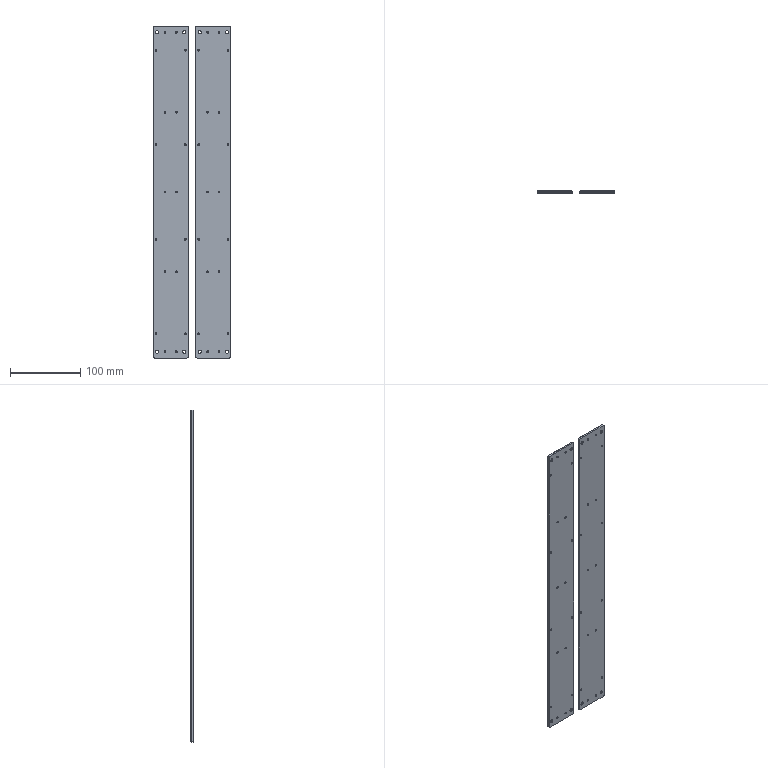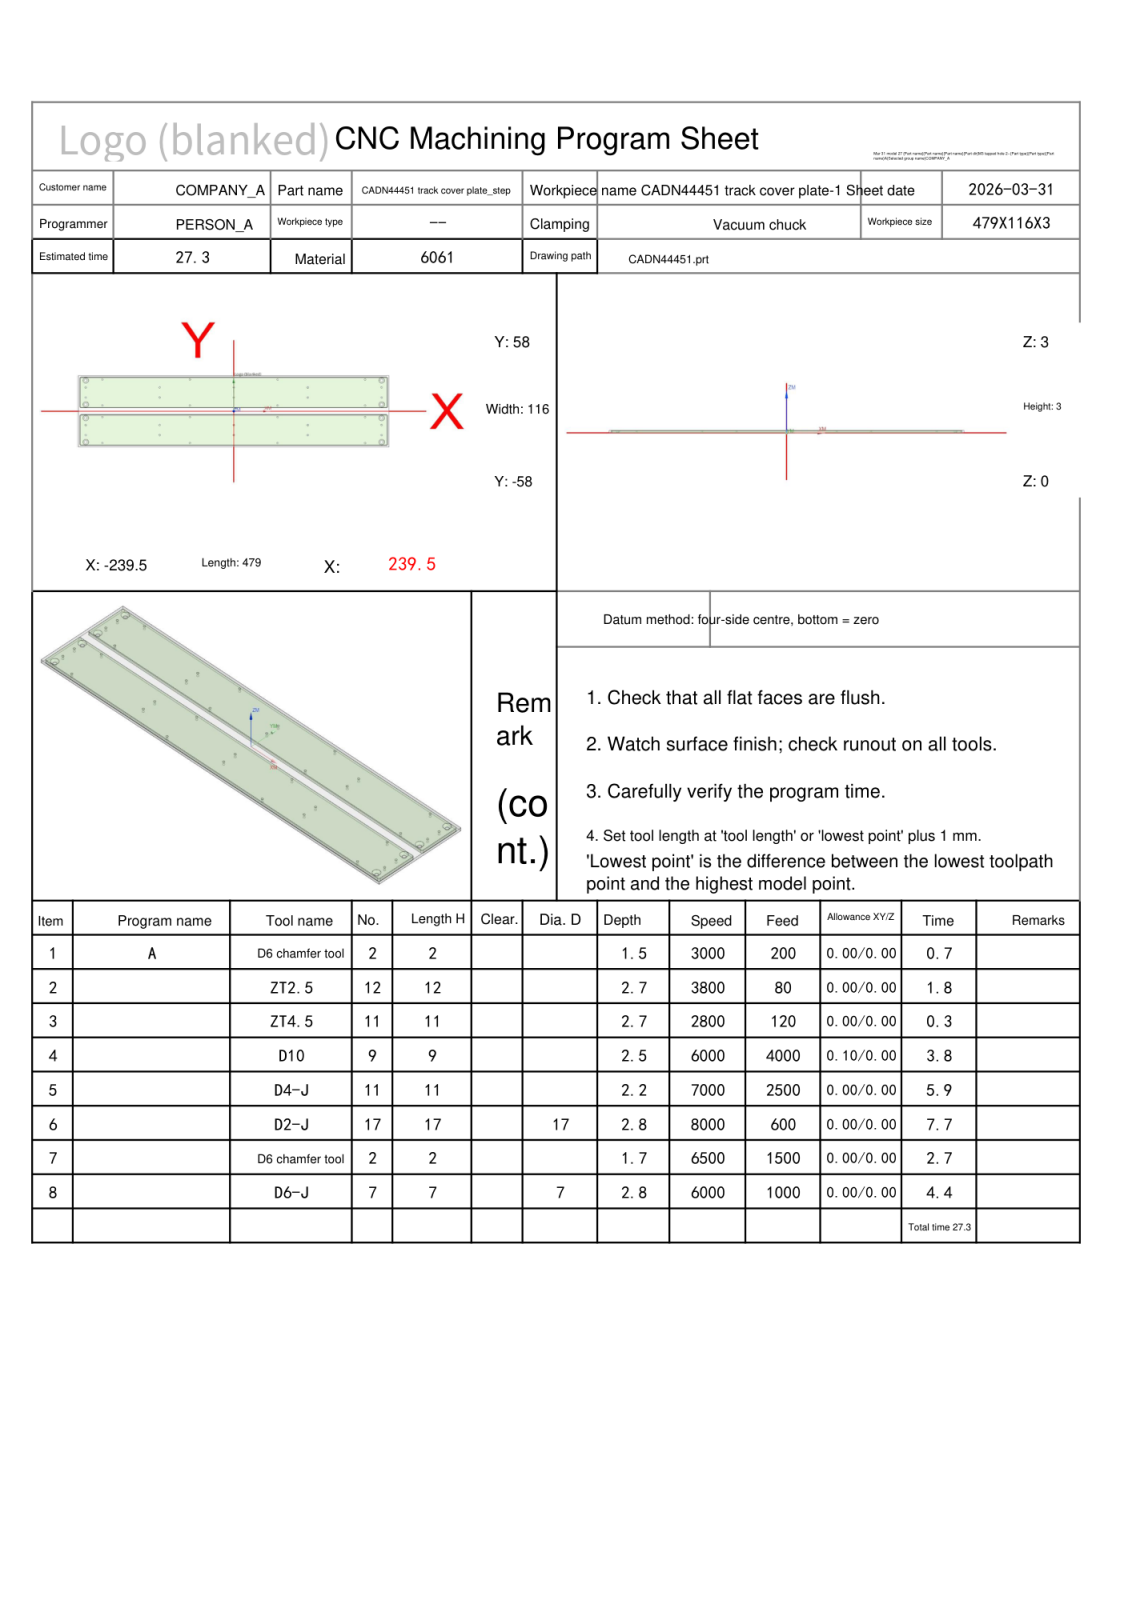NC program | NX | posted by the shop | part box 111 x 3 x 474 mm
Lines 279 to 1191 of 17996:
N5 T11 M06
(D4-J  D=4. R=0. H=11 ce=0.00 di=0.00)
G00 G90 G54 X226.061 Y51.525 M03 S7000
G43 H11 Z23.
M08
Z4.5
G01 X225.989 Y51.441 Z4.494 F2500.
X225.822 Y51.174 Z4.478
X225.661 Y50.807 Z4.457
X225.561 Y50.419 Z4.436
X225.526 Y50.019 Z4.415
X225.555 Y49.619 Z4.394
X225.649 Y49.229 Z4.373
X225.804 Y48.859 Z4.352
X226.017 Y48.52 Z4.331
X226.283 Y48.219 Z4.31
X226.593 Y47.965 Z4.289
X226.94 Y47.764 Z4.268
X227.232 Y47.648 Z4.251
X227.53 Y47.571 Z4.235
X227.835 Y47.531 Z4.219
X228.143 Y47.53 Z4.203
X228.455 Y47.568 Z4.186
X228.861 Y47.68 Z4.164
X229.242 Y47.86 Z4.142
X229.587 Y48.102 Z4.12
X229.886 Y48.399 Z4.098
X230.131 Y48.742 Z4.076
X230.313 Y49.121 Z4.054
X230.429 Y49.526 Z4.032
X230.474 Y49.945 Z4.01
X230.447 Y50.366 Z3.988
X230.35 Y50.776 Z3.965
X230.184 Y51.163 Z3.943
X230.019 Y51.431 Z3.927
X229.734 Y51.766 Z3.904
X229.393 Y52.045 Z3.881
X229.009 Y52.259 Z3.858
X228.592 Y52.402 Z3.835
X228.157 Y52.469 Z3.812
X227.843 Z3.795
X227.41 Y52.403 Z3.772
X226.996 Y52.262 Z3.749
X226.613 Y52.049 Z3.726
X226.274 Y51.773 Z3.703
X225.989 Y51.441 Z3.68
X225.822 Y51.174 Z3.664
X225.661 Y50.807 Z3.643
X225.561 Y50.419 Z3.622
X225.526 Y50.019 Z3.601
X225.555 Y49.619 Z3.58
X225.649 Y49.229 Z3.559
X225.804 Y48.859 Z3.538
X226.017 Y48.52 Z3.517
X226.283 Y48.219 Z3.496
X226.593 Y47.965 Z3.475
X226.94 Y47.764 Z3.454
X227.232 Y47.648 Z3.437
X227.53 Y47.571 Z3.421
X227.835 Y47.531 Z3.405
X228.143 Y47.53 Z3.389
X228.455 Y47.568 Z3.372
X228.861 Y47.68 Z3.35
X229.242 Y47.86 Z3.328
X229.587 Y48.102 Z3.306
X229.886 Y48.399 Z3.284
X230.131 Y48.742 Z3.262
X230.313 Y49.121 Z3.24
X230.429 Y49.526 Z3.218
X230.474 Y49.945 Z3.196
X230.447 Y50.366 Z3.174
X230.35 Y50.776 Z3.152
X230.184 Y51.163 Z3.129
X230.019 Y51.431 Z3.113
X229.734 Y51.766 Z3.09
X229.393 Y52.045 Z3.067
X229.009 Y52.259 Z3.044
X228.592 Y52.402 Z3.021
X228.157 Y52.469 Z2.998
X228. Z2.989
G03 X225.531 Y50. I0.0 J-2.469
X228. Y47.531 I2.469 J0.0
X230.469 Y50. I0.0 J2.469
X228. Y52.469 I-2.469 J0.0
G01 X227.94 Y52.463 Z2.984
X227.879 Y52.456 Z2.979
G03 X225.541 Y50. I.121 J-2.456
X228. Y47.541 I2.459 J0.0
X230.459 Y50. I0.0 J2.459
X228. Y52.459 I-2.459 J0.0
G01 X227.94 Y52.453 Z2.973
X227.879 Y52.445 Z2.968
G03 X225.552 Y50. I.121 J-2.445
X228. Y47.552 I2.448 J0.0
X230.448 Y50. I0.0 J2.448
X228. Y52.448 I-2.448 J0.0
G01 X227.94 Y52.442 Z2.963
X227.879 Y52.435 Z2.958
G03 X225.562 Y50. I.121 J-2.435
X228. Y47.562 I2.438 J0.0
X230.438 Y50. I0.0 J2.438
X228. Y52.438 I-2.438 J0.0
G01 X227.94 Y52.432 Z2.952
X227.879 Y52.424 Z2.947
G03 X225.573 Y50. I.121 J-2.424
X228. Y47.573 I2.427 J0.0
X230.427 Y50. I0.0 J2.427
X228. Y52.427 I-2.427 J0.0
G01 X227.94 Y52.421 Z2.942
X227.879 Y52.413 Z2.936
G03 X225.584 Y50. I.121 J-2.413
X228. Y47.584 I2.416 J0.0
X230.416 Y50. I0.0 J2.416
X228. Y52.416 I-2.416 J0.0
G01 X227.94 Y52.41 Z2.931
X227.879 Y52.403 Z2.926
G03 X225.594 Y50. I.121 J-2.403
X228. Y47.594 I2.406 J0.0
X230.406 Y50. I0.0 J2.406
X228. Y52.406 I-2.406 J0.0
G01 X227.94 Y52.4 Z2.92
X227.879 Y52.392 Z2.915
G03 X225.605 Y50. I.121 J-2.392
X228. Y47.605 I2.395 J0.0
X230.395 Y50. I0.0 J2.395
X228. Y52.395 I-2.395 J0.0
G01 X227.94 Y52.389 Z2.91
X227.879 Y52.381 Z2.905
G03 X225.615 Y50. I.121 J-2.381
X228. Y47.615 I2.385 J0.0
X230.385 Y50. I0.0 J2.385
X228. Y52.385 I-2.385 J0.0
G01 X227.94 Y52.378 Z2.899
X227.879 Y52.371 Z2.894
G03 X225.626 Y50. I.121 J-2.371
X228. Y47.626 I2.374 J0.0
X230.374 Y50. I0.0 J2.374
X228. Y52.374 I-2.374 J0.0
G01 X227.94 Y52.368 Z2.889
X227.879 Y52.36 Z2.883
G03 X225.637 Y50. I.121 J-2.36
X228. Y47.637 I2.363 J0.0
X230.363 Y50. I0.0 J2.363
X228. Y52.363 I-2.363 J0.0
G01 X227.94 Y52.357 Z2.878
X227.879 Y52.35 Z2.873
G03 X225.647 Y50. I.121 J-2.35
X228. Y47.647 I2.353 J0.0
X230.353 Y50. I0.0 J2.353
X228. Y52.353 I-2.353 J0.0
G01 X227.94 Y52.347 Z2.867
X227.879 Y52.339 Z2.862
G03 X225.658 Y50. I.121 J-2.339
X228. Y47.658 I2.342 J0.0
X230.342 Y50. I0.0 J2.342
X228. Y52.342 I-2.342 J0.0
G01 X227.94 Y52.336 Z2.857
X227.879 Y52.328 Z2.852
G03 X225.668 Y50. I.121 J-2.328
X228. Y47.668 I2.332 J0.0
X230.332 Y50. I0.0 J2.332
X228. Y52.332 I-2.332 J0.0
G01 X227.94 Y52.325 Z2.846
X227.879 Y52.318 Z2.841
G03 X225.679 Y50. I.121 J-2.318
X228. Y47.679 I2.321 J0.0
X230.321 Y50. I0.0 J2.321
X228. Y52.321 I-2.321 J0.0
G01 X227.94 Y52.315 Z2.836
X227.879 Y52.307 Z2.83
G03 X225.69 Y50. I.121 J-2.307
X228. Y47.69 I2.31 J0.0
X230.31 Y50. I0.0 J2.31
X228. Y52.31 I-2.31 J0.0
G01 X227.94 Y52.304 Z2.825
X227.879 Y52.297 Z2.82
G03 X225.7 Y50. I.121 J-2.297
X228. Y47.7 I2.3 J0.0
X230.3 Y50. I0.0 J2.3
X228. Y52.3 I-2.3 J0.0
G01 X227.94 Y52.294 Z2.814
X227.879 Y52.286 Z2.809
G03 X225.711 Y50. I.121 J-2.286
X228. Y47.711 I2.289 J0.0
X230.289 Y50. I0.0 J2.289
X228. Y52.289 I-2.289 J0.0
G01 X227.94 Y52.283 Z2.804
X227.879 Y52.275 Z2.798
G03 X225.722 Y50. I.121 J-2.275
X228. Y47.722 I2.278 J0.0
X230.278 Y50. I0.0 J2.278
X228. Y52.278 I-2.278 J0.0
G01 X227.94 Y52.272 Z2.793
X227.879 Y52.265 Z2.788
G03 X225.732 Y50. I.121 J-2.265
X228. Y47.732 I2.268 J0.0
X230.268 Y50. I0.0 J2.268
X228. Y52.268 I-2.268 J0.0
G01 X227.94 Y52.262 Z2.783
X227.879 Y52.254 Z2.777
G03 X225.743 Y50. I.121 J-2.254
X228. Y47.743 I2.257 J0.0
X230.257 Y50. I0.0 J2.257
X228. Y52.257 I-2.257 J0.0
G01 X227.94 Y52.251 Z2.772
X227.879 Y52.243 Z2.767
G03 X225.753 Y50. I.121 J-2.243
X228. Y47.753 I2.247 J0.0
X230.247 Y50. I0.0 J2.247
X228. Y52.247 I-2.247 J0.0
G01 X227.94 Y52.241 Z2.761
X227.879 Y52.233 Z2.756
G03 X225.764 Y50. I.121 J-2.233
X228. Y47.764 I2.236 J0.0
X230.236 Y50. I0.0 J2.236
X228. Y52.236 I-2.236 J0.0
G01 X227.94 Y52.23 Z2.751
X227.879 Y52.222 Z2.745
G03 X225.775 Y50. I.121 J-2.222
X228. Y47.775 I2.225 J0.0
X230.225 Y50. I0.0 J2.225
X228. Y52.225 I-2.225 J0.0
G01 X227.94 Y52.219 Z2.74
X227.879 Y52.212 Z2.735
G03 X225.785 Y50. I.121 J-2.212
X228. Y47.785 I2.215 J0.0
X230.215 Y50. I0.0 J2.215
X228. Y52.215 I-2.215 J0.0
G01 X227.94 Y52.209 Z2.73
X227.879 Y52.201 Z2.724
G03 X225.796 Y50. I.121 J-2.201
X228. Y47.796 I2.204 J0.0
X230.204 Y50. I0.0 J2.204
X228. Y52.204 I-2.204 J0.0
G01 X227.94 Y52.198 Z2.719
X227.879 Y52.19 Z2.714
G03 X225.806 Y50. I.121 J-2.19
X228. Y47.806 I2.194 J0.0
X230.194 Y50. I0.0 J2.194
X228. Y52.194 I-2.194 J0.0
G01 X227.94 Y52.187 Z2.708
X227.879 Y52.18 Z2.703
G03 X225.817 Y50. I.121 J-2.18
X228. Y47.817 I2.183 J0.0
X230.183 Y50. I0.0 J2.183
X228. Y52.183 I-2.183 J0.0
G01 X227.94 Y52.177 Z2.698
X227.879 Y52.169 Z2.692
G03 X225.828 Y50. I.121 J-2.169
X228. Y47.828 I2.172 J0.0
X230.172 Y50. I0.0 J2.172
X228. Y52.172 I-2.172 J0.0
G01 X227.94 Y52.166 Z2.687
X227.879 Y52.158 Z2.682
G03 X225.838 Y50. I.121 J-2.158
X228. Y47.838 I2.162 J0.0
X230.162 Y50. I0.0 J2.162
X228. Y52.162 I-2.162 J0.0
G01 X227.94 Y52.156 Z2.676
X227.879 Y52.148 Z2.671
G03 X225.849 Y50. I.121 J-2.148
X228. Y47.849 I2.151 J0.0
X230.151 Y50. I0.0 J2.151
X228. Y52.151 I-2.151 J0.0
G01 X227.94 Y52.145 Z2.666
X227.879 Y52.137 Z2.661
G03 X225.859 Y50. I.121 J-2.137
X228. Y47.859 I2.141 J0.0
X230.141 Y50. I0.0 J2.141
X228. Y52.141 I-2.141 J0.0
G01 X227.94 Y52.134 Z2.655
X227.879 Y52.127 Z2.65
G03 X225.87 Y50. I.121 J-2.127
X228. Y47.87 I2.13 J0.0
X230.13 Y50. I0.0 J2.13
X228. Y52.13 I-2.13 J0.0
G01 X227.94 Y52.124 Z2.645
X227.879 Y52.116 Z2.639
G03 X225.881 Y50. I.121 J-2.116
X228. Y47.881 I2.119 J0.0
X230.119 Y50. I0.0 J2.119
X228. Y52.119 I-2.119 J0.0
G01 X227.94 Y52.113 Z2.634
X227.879 Y52.105 Z2.629
G03 X225.891 Y50. I.121 J-2.105
X228. Y47.891 I2.109 J0.0
X230.109 Y50. I0.0 J2.109
X228. Y52.109 I-2.109 J0.0
G01 X227.94 Y52.103 Z2.623
X227.879 Y52.095 Z2.618
G03 X225.902 Y50. I.121 J-2.095
X228. Y47.902 I2.098 J0.0
X230.098 Y50. I0.0 J2.098
X228. Y52.098 I-2.098 J0.0
G01 X227.94 Y52.092 Z2.613
X227.879 Y52.084 Z2.608
G03 X225.912 Y50. I.121 J-2.084
X228. Y47.912 I2.088 J0.0
X230.088 Y50. I0.0 J2.088
X228. Y52.088 I-2.088 J0.0
G01 X227.94 Y52.081 Z2.602
X227.879 Y52.073 Z2.597
G03 X225.923 Y50. I.121 J-2.073
X228. Y47.923 I2.077 J0.0
X230.077 Y50. I0.0 J2.077
X228. Y52.077 I-2.077 J0.0
G01 X227.94 Y52.071 Z2.592
X227.879 Y52.063 Z2.586
G03 X225.934 Y50. I.121 J-2.063
X228. Y47.934 I2.066 J0.0
X230.066 Y50. I0.0 J2.066
X228. Y52.066 I-2.066 J0.0
G01 X227.94 Y52.06 Z2.581
X227.879 Y52.052 Z2.576
G03 X225.944 Y50. I.121 J-2.052
X228. Y47.944 I2.056 J0.0
X230.056 Y50. I0.0 J2.056
X228. Y52.056 I-2.056 J0.0
G01 X227.94 Y52.05 Z2.57
X227.879 Y52.042 Z2.565
G03 X225.955 Y50. I.121 J-2.042
X228. Y47.955 I2.045 J0.0
X230.045 Y50. I0.0 J2.045
X228. Y52.045 I-2.045 J0.0
G01 X227.94 Y52.039 Z2.56
X227.879 Y52.031 Z2.555
G03 X225.965 Y50. I.121 J-2.031
X228. Y47.965 I2.035 J0.0
X230.035 Y50. I0.0 J2.035
X228. Y52.035 I-2.035 J0.0
G01 X227.94 Y52.028 Z2.549
X227.879 Y52.02 Z2.544
G03 X225.976 Y50. I.121 J-2.02
X228. Y47.976 I2.024 J0.0
X230.024 Y50. I0.0 J2.024
X228. Y52.024 I-2.024 J0.0
G01 X227.94 Y52.018 Z2.539
X227.879 Y52.01 Z2.533
G03 X225.987 Y50. I.121 J-2.01
X228. Y47.987 I2.013 J0.0
X230.013 Y50. I0.0 J2.013
X228. Y52.013 I-2.013 J0.0
G01 X227.94 Y52.007 Z2.528
X227.879 Y51.999 Z2.523
G03 X225.997 Y50. I.121 J-1.999
X228. Y47.997 I2.003 J0.0
X230.003 Y50. I0.0 J2.003
X228. Y52.003 I-2.003 J0.0
G01 X227.94 Y51.996 Z2.517
X227.879 Y51.988 Z2.512
G03 X226.008 Y50. I.121 J-1.988
X228. Y48.008 I1.992 J0.0
X229.992 Y50. I0.0 J1.992
X228. Y51.992 I-1.992 J0.0
G01 X227.94 Y51.986 Z2.507
X227.879 Y51.978 Z2.501
G03 X226.019 Y50. I.121 J-1.978
X228. Y48.019 I1.981 J0.0
X229.981 Y50. I0.0 J1.981
X228. Y51.981 I-1.981 J0.0
G01 X227.94 Y51.975 Z2.496
X227.879 Y51.967 Z2.491
G03 X226.029 Y50. I.121 J-1.967
X228. Y48.029 I1.971 J0.0
X229.971 Y50. I0.0 J1.971
X228. Y51.971 I-1.971 J0.0
G01 X227.94 Y51.965 Z2.486
X227.879 Y51.957 Z2.48
G03 X226.04 Y50. I.121 J-1.957
X228. Y48.04 I1.96 J0.0
X229.96 Y50. I0.0 J1.96
X228. Y51.96 I-1.96 J0.0
G01 X227.94 Y51.954 Z2.475
X227.879 Y51.946 Z2.47
G03 X226.05 Y50. I.121 J-1.946
X228. Y48.05 I1.95 J0.0
X229.95 Y50. I0.0 J1.95
X228. Y51.95 I-1.95 J0.0
G01 X227.94 Y51.943 Z2.464
X227.88 Y51.935 Z2.459
G03 X226.061 Y50. I.12 J-1.935
X228. Y48.061 I1.939 J0.0
X229.939 Y50. I0.0 J1.939
X228. Y51.939 I-1.939 J0.0
G01 X227.94 Y51.933 Z2.454
X227.88 Y51.925 Z2.448
G03 X226.072 Y50. I.12 J-1.925
X228. Y48.072 I1.928 J0.0
X229.928 Y50. I0.0 J1.928
X228. Y51.928 I-1.928 J0.0
G01 X227.94 Y51.922 Z2.443
X227.88 Y51.914 Z2.438
G03 X226.082 Y50. I.12 J-1.914
X228. Y48.082 I1.918 J0.0
X229.918 Y50. I0.0 J1.918
X228. Y51.918 I-1.918 J0.0
G01 X227.94 Y51.912 Z2.433
X227.88 Y51.903 Z2.427
G03 X226.093 Y50. I.12 J-1.903
X228. Y48.093 I1.907 J0.0
X229.907 Y50. I0.0 J1.907
X228. Y51.907 I-1.907 J0.0
G01 X227.94 Y51.901 Z2.422
X227.88 Y51.893 Z2.417
G03 X226.103 Y50. I.12 J-1.893
X228. Y48.103 I1.897 J0.0
X229.897 Y50. I0.0 J1.897
X228. Y51.897 I-1.897 J0.0
G01 X227.94 Y51.89 Z2.411
X227.88 Y51.882 Z2.406
G03 X226.114 Y50. I.12 J-1.882
X228. Y48.114 I1.886 J0.0
X229.886 Y50. I0.0 J1.886
X228. Y51.886 I-1.886 J0.0
G01 X227.94 Y51.88 Z2.401
X227.88 Y51.872 Z2.395
G03 X226.125 Y50. I.12 J-1.872
X228. Y48.125 I1.875 J0.0
X229.875 Y50. I0.0 J1.875
X228. Y51.875 I-1.875 J0.0
G01 X227.94 Y51.869 Z2.39
X227.88 Y51.861 Z2.385
G03 X226.135 Y50. I.12 J-1.861
X228. Y48.135 I1.865 J0.0
X229.865 Y50. I0.0 J1.865
X228. Y51.865 I-1.865 J0.0
G01 X227.94 Y51.859 Z2.38
X227.88 Y51.85 Z2.374
G03 X226.146 Y50. I.12 J-1.85
X228. Y48.146 I1.854 J0.0
X229.854 Y50. I0.0 J1.854
X228. Y51.854 I-1.854 J0.0
G01 X227.94 Y51.848 Z2.369
X227.88 Y51.84 Z2.364
G03 X226.156 Y50. I.12 J-1.84
X228. Y48.156 I1.844 J0.0
X229.844 Y50. I0.0 J1.844
X228. Y51.844 I-1.844 J0.0
G01 X227.94 Y51.837 Z2.358
X227.88 Y51.829 Z2.353
G03 X226.167 Y50. I.12 J-1.829
X228. Y48.167 I1.833 J0.0
X229.833 Y50. I0.0 J1.833
X228. Y51.833 I-1.833 J0.0
G01 X227.94 Y51.827 Z2.348
X227.88 Y51.818 Z2.342
G03 X226.178 Y50. I.12 J-1.818
X228. Y48.178 I1.822 J0.0
X229.822 Y50. I0.0 J1.822
X228. Y51.822 I-1.822 J0.0
G01 X227.94 Y51.816 Z2.337
X227.88 Y51.808 Z2.332
G03 X226.188 Y50. I.12 J-1.808
X228. Y48.188 I1.812 J0.0
X229.812 Y50. I0.0 J1.812
X228. Y51.812 I-1.812 J0.0
G01 X227.94 Y51.805 Z2.326
X227.88 Y51.797 Z2.321
G03 X226.199 Y50. I.12 J-1.797
X228. Y48.199 I1.801 J0.0
X229.801 Y50. I0.0 J1.801
X228. Y51.801 I-1.801 J0.0
G01 X227.94 Y51.795 Z2.316
X227.88 Y51.787 Z2.311
G03 X226.209 Y50. I.12 J-1.787
X228. Y48.209 I1.791 J0.0
X229.791 Y50. I0.0 J1.791
X228. Y51.791 I-1.791 J0.0
G01 X227.94 Y51.784 Z2.305
X227.88 Y51.776 Z2.3
G03 X226.22 Y50. I.12 J-1.776
X228. Y48.22 I1.78 J0.0
X229.78 Y50. I0.0 J1.78
X228. Y51.78 I-1.78 J0.0
G01 X227.94 Y51.774 Z2.295
X227.88 Y51.765 Z2.289
G03 X226.231 Y50. I.12 J-1.765
X228. Y48.231 I1.769 J0.0
X229.769 Y50. I0.0 J1.769
X228. Y51.769 I-1.769 J0.0
G01 X227.94 Y51.763 Z2.284
X227.88 Y51.755 Z2.279
G03 X226.241 Y50. I.12 J-1.755
X228. Y48.241 I1.759 J0.0
X229.759 Y50. I0.0 J1.759
X228. Y51.759 I-1.759 J0.0
G01 X227.94 Y51.752 Z2.273
X227.88 Y51.744 Z2.268
G03 X226.252 Y50. I.12 J-1.744
X228. Y48.252 I1.748 J0.0
X229.748 Y50. I0.0 J1.748
X228. Y51.748 I-1.748 J0.0
G01 X227.94 Y51.742 Z2.263
X227.88 Y51.733 Z2.258
G03 X226.262 Y50. I.12 J-1.733
X228. Y48.262 I1.738 J0.0
X229.738 Y50. I0.0 J1.738
X228. Y51.738 I-1.738 J0.0
G01 X227.94 Y51.731 Z2.252
X227.88 Y51.723 Z2.247
G03 X226.273 Y50. I.12 J-1.723
X228. Y48.273 I1.727 J0.0
X229.727 Y50. I0.0 J1.727
X228. Y51.727 I-1.727 J0.0
G01 X227.94 Y51.721 Z2.242
X227.88 Y51.712 Z2.236
G03 X226.284 Y50. I.12 J-1.712
X228. Y48.284 I1.716 J0.0
X229.716 Y50. I0.0 J1.716
X228. Y51.716 I-1.716 J0.0
G01 X227.94 Y51.71 Z2.231
X227.88 Y51.701 Z2.226
G03 X226.294 Y50. I.12 J-1.701
X228. Y48.294 I1.706 J0.0
X229.706 Y50. I0.0 J1.706
X228. Y51.706 I-1.706 J0.0
G01 X227.94 Y51.699 Z2.22
X227.88 Y51.691 Z2.215
G03 X226.305 Y50. I.12 J-1.691
X228. Y48.305 I1.695 J0.0
X229.695 Y50. I0.0 J1.695
X228. Y51.695 I-1.695 J0.0
G01 X227.94 Y51.689 Z2.21
X227.88 Y51.68 Z2.205
G03 X226.315 Y50. I.12 J-1.68
X228. Y48.315 I1.685 J0.0
X229.685 Y50. I0.0 J1.685
X228. Y51.685 I-1.685 J0.0
G01 X227.94 Y51.678 Z2.199
X227.88 Y51.67 Z2.194
G03 X226.326 Y50. I.12 J-1.67
X228. Y48.326 I1.674 J0.0
X229.674 Y50. I0.0 J1.674
X228. Y51.674 I-1.674 J0.0
G01 X227.94 Y51.668 Z2.189
X227.88 Y51.659 Z2.183
G03 X226.337 Y50. I.12 J-1.659
X228. Y48.337 I1.663 J0.0
X229.663 Y50. I0.0 J1.663
X228. Y51.663 I-1.663 J0.0
G01 X227.94 Y51.657 Z2.178
X227.88 Y51.648 Z2.173
G03 X226.347 Y50. I.12 J-1.648
X228. Y48.347 I1.653 J0.0
X229.653 Y50. I0.0 J1.653
X228. Y51.653 I-1.653 J0.0
G01 X227.94 Y51.646 Z2.167
X227.88 Y51.638 Z2.162
G03 X226.358 Y50. I.12 J-1.638
X228. Y48.358 I1.642 J0.0
X229.642 Y50. I0.0 J1.642
X228. Y51.642 I-1.642 J0.0
G01 X227.94 Y51.636 Z2.157
X227.88 Y51.627 Z2.151
G03 X226.369 Y50. I.12 J-1.627
X228. Y48.369 I1.631 J0.0
X229.631 Y50. I0.0 J1.631
X228. Y51.631 I-1.631 J0.0
G01 X227.94 Y51.625 Z2.146
X227.88 Y51.616 Z2.141
G03 X226.379 Y50. I.12 J-1.616
X228. Y48.379 I1.621 J0.0
X229.621 Y50. I0.0 J1.621
X228. Y51.621 I-1.621 J0.0
G01 X227.94 Y51.614 Z2.136
X227.88 Y51.606 Z2.13
G03 X226.39 Y50. I.12 J-1.606
X228. Y48.39 I1.61 J0.0
X229.61 Y50. I0.0 J1.61
X228. Y51.61 I-1.61 J0.0
G01 X227.94 Y51.604 Z2.125
X227.88 Y51.595 Z2.12
G03 X226.4 Y50. I.12 J-1.595
X228. Y48.4 I1.6 J0.0
X229.6 Y50. I0.0 J1.6
X228. Y51.6 I-1.6 J0.0
G01 X227.94 Y51.593 Z2.114
X227.88 Y51.584 Z2.109
G03 X226.411 Y50. I.12 J-1.584
X228. Y48.411 I1.589 J0.0
X229.589 Y50. I0.0 J1.589
X228. Y51.589 I-1.589 J0.0
G01 X227.94 Y51.583 Z2.104
X227.88 Y51.574 Z2.098
G03 X226.422 Y50. I.12 J-1.574
X228. Y48.422 I1.578 J0.0
X229.578 Y50. I0.0 J1.578
X228. Y51.578 I-1.578 J0.0
G01 X227.94 Y51.572 Z2.093
X227.88 Y51.563 Z2.088
G03 X226.432 Y50. I.12 J-1.563
X228. Y48.432 I1.568 J0.0
X229.568 Y50. I0.0 J1.568
X228. Y51.568 I-1.568 J0.0
G01 X227.94 Y51.561 Z2.083
X227.88 Y51.553 Z2.077
G03 X226.443 Y50. I.12 J-1.553
X228. Y48.443 I1.557 J0.0
X229.557 Y50. I0.0 J1.557
X228. Y51.557 I-1.557 J0.0
G01 X227.94 Y51.551 Z2.072
X227.88 Y51.542 Z2.067
G03 X226.453 Y50. I.12 J-1.542
X228. Y48.453 I1.547 J0.0
X229.547 Y50. I0.0 J1.547
X228. Y51.547 I-1.547 J0.0
G01 X227.94 Y51.54 Z2.061
X227.88 Y51.531 Z2.056
G03 X226.464 Y50. I.12 J-1.531
X228. Y48.464 I1.536 J0.0
X229.536 Y50. I0.0 J1.536
X228. Y51.536 I-1.536 J0.0
G01 X227.94 Y51.53 Z2.051
X227.88 Y51.521 Z2.045
G03 X226.475 Y50. I.12 J-1.521
X228. Y48.475 I1.525 J0.0
X229.525 Y50. I0.0 J1.525
X228. Y51.525 I-1.525 J0.0
G01 X227.94 Y51.519 Z2.04
X227.88 Y51.51 Z2.035
G03 X226.485 Y50. I.12 J-1.51
X228. Y48.485 I1.515 J0.0
X229.515 Y50. I0.0 J1.515
X228. Y51.515 I-1.515 J0.0
G01 X227.94 Y51.508 Z2.029
X227.88 Y51.499 Z2.024
G03 X226.496 Y50. I.12 J-1.499
X228. Y48.496 I1.504 J0.0
X229.504 Y50. I0.0 J1.504
X228. Y51.504 I-1.504 J0.0
G01 X227.94 Y51.498 Z2.019
X227.88 Y51.489 Z2.014
G03 X226.506 Y50. I.12 J-1.489
X228. Y48.506 I1.494 J0.0
X229.494 Y50. I0.0 J1.494
X228. Y51.494 I-1.494 J0.0
G01 X227.94 Y51.487 Z2.008
X227.88 Y51.478 Z2.003
G03 X226.517 Y50. I.12 J-1.478
X228. Y48.517 I1.483 J0.0
X229.483 Y50. I0.0 J1.483
X228. Y51.483 I-1.483 J0.0
G01 X227.94 Y51.476 Z1.998
X227.88 Y51.467 Z1.992
G03 X226.528 Y50. I.12 J-1.467
X228. Y48.528 I1.472 J0.0
X229.472 Y50. I0.0 J1.472
X228. Y51.472 I-1.472 J0.0
G01 X227.94 Y51.466 Z1.987
X227.88 Y51.457 Z1.982
G03 X226.538 Y50. I.12 J-1.457
X228. Y48.538 I1.462 J0.0
X229.462 Y50. I0.0 J1.462
X228. Y51.462 I-1.462 J0.0
G01 X227.94 Y51.455 Z1.976
X227.88 Y51.446 Z1.971
G03 X226.549 Y50. I.12 J-1.446
X228. Y48.549 I1.451 J0.0
X229.451 Y50. I0.0 J1.451
X228. Y51.451 I-1.451 J0.0
G01 X227.94 Y51.445 Z1.966
X227.88 Y51.436 Z1.961
G03 X226.559 Y50. I.12 J-1.436
X228. Y48.559 I1.441 J0.0
X229.441 Y50. I0.0 J1.441
X228. Y51.441 I-1.441 J0.0
G01 X227.94 Y51.434 Z1.955
X227.88 Y51.425 Z1.95
G03 X226.57 Y50. I.12 J-1.425
X228. Y48.57 I1.43 J0.0
X229.43 Y50. I0.0 J1.43
X228. Y51.43 I-1.43 J0.0
G01 X227.94 Y51.423 Z1.945
X227.88 Y51.414 Z1.939
G03 X226.581 Y50. I.12 J-1.414
X228. Y48.581 I1.419 J0.0
X229.419 Y50. I0.0 J1.419
X228. Y51.419 I-1.419 J0.0
G01 X227.94 Y51.413 Z1.934
X227.88 Y51.404 Z1.929
G03 X226.591 Y50. I.12 J-1.404
X228. Y48.591 I1.409 J0.0
X229.409 Y50. I0.0 J1.409
X228. Y51.409 I-1.409 J0.0
G01 X227.94 Y51.402 Z1.923
X227.88 Y51.393 Z1.918
G03 X226.602 Y50. I.12 J-1.393
X228. Y48.602 I1.398 J0.0
X229.398 Y50. I0.0 J1.398
X228. Y51.398 I-1.398 J0.0
G01 X227.94 Y51.392 Z1.913
X227.88 Y51.382 Z1.908
G03 X226.612 Y50. I.12 J-1.382
X228. Y48.612 I1.388 J0.0
X229.388 Y50. I0.0 J1.388
X228. Y51.388 I-1.388 J0.0
G01 X227.94 Y51.381 Z1.902
X227.88 Y51.372 Z1.897
G03 X226.623 Y50. I.12 J-1.372
X228. Y48.623 I1.377 J0.0
X229.377 Y50. I0.0 J1.377
X228. Y51.377 I-1.377 J0.0
G01 X227.94 Y51.37 Z1.892
X227.88 Y51.361 Z1.886
G03 X226.634 Y50. I.12 J-1.361
X228. Y48.634 I1.366 J0.0
X229.366 Y50. I0.0 J1.366
X228. Y51.366 I-1.366 J0.0
G01 X227.94 Y51.36 Z1.881
X227.88 Y51.35 Z1.876
G03 X226.644 Y50. I.12 J-1.35
X228. Y48.644 I1.356 J0.0
X229.356 Y50. I0.0 J1.356
X228. Y51.356 I-1.356 J0.0
G01 X227.94 Y51.349 Z1.87
X227.88 Y51.34 Z1.865
G03 X226.655 Y50. I.12 J-1.34
X228. Y48.655 I1.345 J0.0
X229.345 Y50. I0.0 J1.345
X228. Y51.345 I-1.345 J0.0
G01 X227.94 Y51.338 Z1.86
X227.88 Y51.329 Z1.854
G03 X226.666 Y50. I.12 J-1.329
X228. Y48.666 I1.334 J0.0
X229.334 Y50. I0.0 J1.334
X228. Y51.334 I-1.334 J0.0
G01 X227.94 Y51.328 Z1.849
X227.88 Y51.318 Z1.844
G03 X226.676 Y50. I.12 J-1.318
X228. Y48.676 I1.324 J0.0
X229.324 Y50. I0.0 J1.324
X228. Y51.324 I-1.324 J0.0
G01 X227.94 Y51.317 Z1.839
X227.88 Y51.308 Z1.833
G03 X226.687 Y50. I.12 J-1.308
X228. Y48.687 I1.313 J0.0
X229.313 Y50. I0.0 J1.313
X228. Y51.313 I-1.313 J0.0
G01 X227.94 Y51.307 Z1.828
X227.88 Y51.297 Z1.823
G03 X226.697 Y50. I.12 J-1.297
X228. Y48.697 I1.303 J0.0
X229.303 Y50. I0.0 J1.303
X228. Y51.303 I-1.303 J0.0
G01 X227.94 Y51.296 Z1.817
X227.88 Y51.286 Z1.812
G03 X226.708 Y50. I.12 J-1.286
X228. Y48.708 I1.292 J0.0
X229.292 Y50. I0.0 J1.292
X228. Y51.292 I-1.292 J0.0
G01 X227.94 Y51.285 Z1.807
X227.88 Y51.276 Z1.801
G03 X226.719 Y50. I.12 J-1.276
X228. Y48.719 I1.281 J0.0
X229.281 Y50. I0.0 J1.281
X228. Y51.281 I-1.281 J0.0
G01 X227.94 Y51.275 Z1.796
X227.88 Y51.265 Z1.791
G03 X226.729 Y50. I.12 J-1.265
X228. Y48.729 I1.271 J0.0
X229.271 Y50. I0.0 J1.271
X228. Y51.271 I-1.271 J0.0
G01 X227.94 Y51.264 Z1.786
X227.88 Y51.255 Z1.78
G03 X226.74 Y50. I.12 J-1.255
X228. Y48.74 I1.26 J0.0
X229.26 Y50. I0.0 J1.26
X228. Y51.26 I-1.26 J0.0
G01 X227.94 Y51.253 Z1.775
X227.88 Y51.244 Z1.77
G03 X226.75 Y50. I.12 J-1.244
X228. Y48.75 I1.25 J0.0
X229.25 Y50. I0.0 J1.25
X228. Y51.25 I-1.25 J0.0
G01 X227.94 Y51.243 Z1.764
X227.88 Y51.233 Z1.759
G03 X226.761 Y50. I.12 J-1.233
X228. Y48.761 I1.239 J0.0
X229.239 Y50. I0.0 J1.239
X228. Y51.239 I-1.239 J0.0
G01 X227.94 Y51.232 Z1.754
X227.88 Y51.223 Z1.748
G03 X226.772 Y50. I.12 J-1.223
X228. Y48.772 I1.228 J0.0
X229.228 Y50. I0.0 J1.228
X228. Y51.228 I-1.228 J0.0
G01 X227.94 Y51.222 Z1.743
X227.88 Y51.212 Z1.738
G03 X226.782 Y50. I.12 J-1.212
X228. Y48.782 I1.218 J0.0
X229.218 Y50. I0.0 J1.218
X228. Y51.218 I-1.218 J0.0
G01 X227.94 Y51.211 Z1.733
X227.88 Y51.201 Z1.727
G03 X226.793 Y50. I.12 J-1.201
X228. Y48.793 I1.207 J0.0
X229.207 Y50. I0.0 J1.207
X228. Y51.207 I-1.207 J0.0
G01 X227.94 Y51.2 Z1.722
X227.88 Y51.191 Z1.717
G03 X226.803 Y50. I.12 J-1.191
X228. Y48.803 I1.197 J0.0
X229.197 Y50. I0.0 J1.197
X228. Y51.197 I-1.197 J0.0
G01 X227.94 Y51.19 Z1.711
X227.88 Y51.18 Z1.706
G03 X226.814 Y50. I.12 J-1.18
X228. Y48.814 I1.186 J0.0
X229.186 Y50. I0.0 J1.186
X228. Y51.186 I-1.186 J0.0
G01 X227.94 Y51.179 Z1.701
X227.88 Y51.169 Z1.695
G03 X226.825 Y50. I.12 J-1.169
X228. Y48.825 I1.175 J0.0
X229.175 Y50. I0.0 J1.175
X228. Y51.175 I-1.175 J0.0
G01 X227.94 Y51.169 Z1.69
X227.88 Y51.159 Z1.685
G03 X226.835 Y50. I.12 J-1.159
X228. Y48.835 I1.165 J0.0
X229.165 Y50. I0.0 J1.165
X228. Y51.165 I-1.165 J0.0
G01 X227.94 Y51.158 Z1.679
X227.88 Y51.148 Z1.674
G03 X226.846 Y50. I.12 J-1.148
X228. Y48.846 I1.154 J0.0
X229.154 Y50. I0.0 J1.154
X228. Y51.154 I-1.154 J0.0
G01 X227.94 Y51.147 Z1.669
X227.88 Y51.137 Z1.664
G03 X226.856 Y50. I.12 J-1.137
X228. Y48.856 I1.144 J0.0
X229.144 Y50. I0.0 J1.144
X228. Y51.144 I-1.144 J0.0
G01 X227.94 Y51.137 Z1.658
X227.88 Y51.127 Z1.653
G03 X226.867 Y50. I.12 J-1.127
X228. Y48.867 I1.133 J0.0
X229.133 Y50. I0.0 J1.133
X228. Y51.133 I-1.133 J0.0
G01 X227.94 Y51.126 Z1.648
X227.88 Y51.116 Z1.642
G03 X226.878 Y50. I.12 J-1.116
X228. Y48.878 I1.122 J0.0
X229.122 Y50. I0.0 J1.122
X228. Y51.122 I-1.122 J0.0
G01 X227.94 Y51.115 Z1.637
X227.88 Y51.105 Z1.632
G03 X226.888 Y50. I.12 J-1.105
X228. Y48.888 I1.112 J0.0
X229.112 Y50. I0.0 J1.112
X228. Y51.112 I-1.112 J0.0
G01 X227.94 Y51.105 Z1.626
X227.88 Y51.095 Z1.621
G03 X226.899 Y50. I.12 J-1.095
X228. Y48.899 I1.101 J0.0
X229.101 Y50. I0.0 J1.101
X228. Y51.101 I-1.101 J0.0
G01 X227.94 Y51.094 Z1.616
X227.88 Y51.084 Z1.611
G03 X226.909 Y50. I.12 J-1.084
X228. Y48.909 I1.091 J0.0
X229.091 Y50. I0.0 J1.091
X228. Y51.091 I-1.091 J0.0
G01 X227.94 Y51.084 Z1.605
X227.88 Y51.073 Z1.6
G03 X226.92 Y50. I.12 J-1.073
X228. Y48.92 I1.08 J0.0
X229.08 Y50. I0.0 J1.08
X228. Y51.08 I-1.08 J0.0
G01 X227.94 Y51.073 Z1.595
X227.88 Y51.063 Z1.589
G03 X226.931 Y50. I.12 J-1.063
X228. Y48.931 I1.069 J0.0
X229.069 Y50. I0.0 J1.069
X228. Y51.069 I-1.069 J0.0
G01 X227.94 Y51.062 Z1.584
X227.88 Y51.052 Z1.579
G03 X226.941 Y50. I.12 J-1.052
X228. Y48.941 I1.059 J0.0
X229.059 Y50. I0.0 J1.059
X228. Y51.059 I-1.059 J0.0
G01 X227.94 Y51.052 Z1.573
X227.88 Y51.041 Z1.568
G03 X226.952 Y50. I.12 J-1.041
X228. Y48.952 I1.048 J0.0
X229.048 Y50. I0.0 J1.048
X228. Y51.048 I-1.048 J0.0
G01 X227.94 Y51.041 Z1.563
X227.88 Y51.031 Z1.558
G03 X226.962 Y50. I.12 J-1.031
X228. Y48.962 I1.038 J0.0
X229.038 Y50. I0.0 J1.038
X228. Y51.038 I-1.038 J0.0
G01 X227.94 Y51.03 Z1.552
X227.88 Y51.02 Z1.547
G03 X226.973 Y50. I.12 J-1.02
X228. Y48.973 I1.027 J0.0
X229.027 Y50. I0.0 J1.027
X228. Y51.027 I-1.027 J0.0
G01 X227.94 Y51.02 Z1.542
X227.88 Y51.009 Z1.536
G03 X226.984 Y50. I.12 J-1.009
X228. Y48.984 I1.016 J0.0
X229.016 Y50. I0.0 J1.016
X228. Y51.016 I-1.016 J0.0
G01 X227.94 Y51.009 Z1.531
X227.88 Y50.999 Z1.526
G03 X226.994 Y50. I.12 J-.999
X228. Y48.994 I1.006 J0.0
X229.006 Y50. I0.0 J1.006
X228. Y51.006 I-1.006 J0.0
G01 X227.94 Y50.999 Z1.52